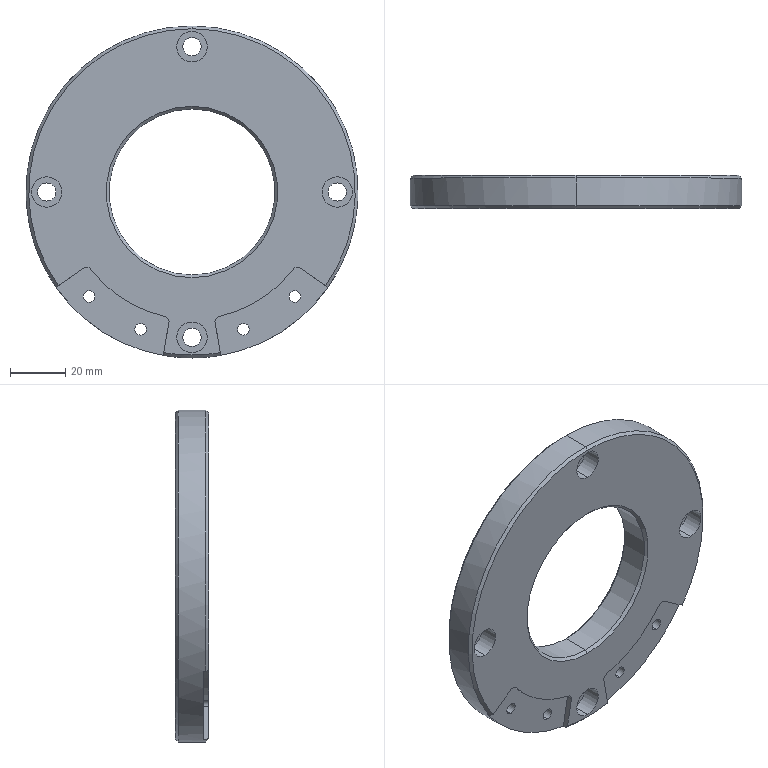Part | SolidWorks | features HoleWzd 2, Chamfer 1, Extrusion 1, Fillet 1, ICE 1 | 1 solid | 55 faces | box 120 x 12 x 120 mm | volume 95094 mm3 | cylinder 34 | plane 12 | cone 9 | commonest cylinder face diameters 4.2 x8 6.6 x8 11 x8 4 x4 60 x2 92 x2